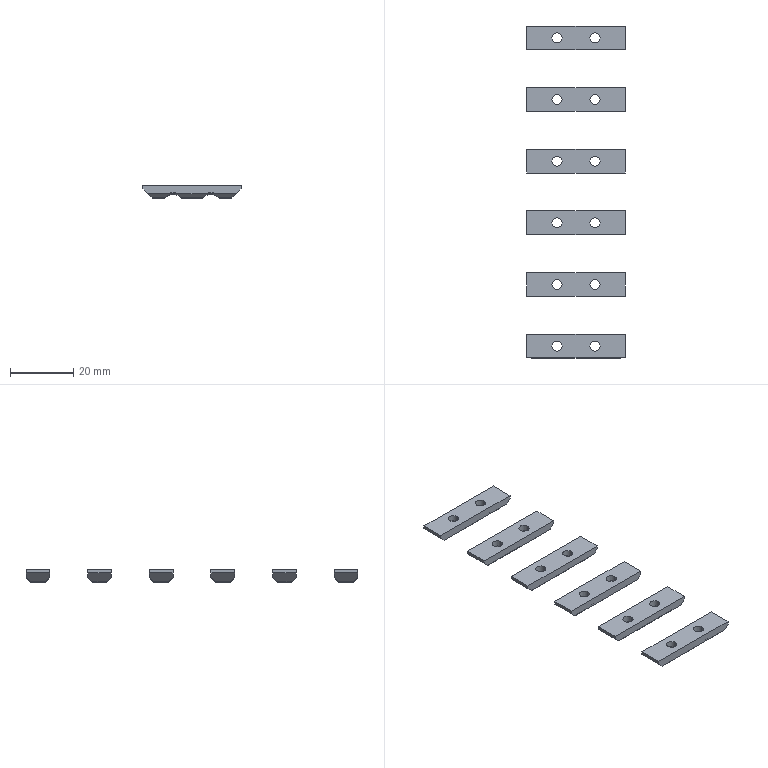NC program | NX | posted with a generic post | part box 31 x 105 x 4 mm
Lines 12431 to 12738 of 12738:
(ZLEVEL_PROFILE_1_COPY , TOOL : D10JING)
N24788 T14 M6
N24790 G54
N24792 G17 G0 G90 X44.871 Y20.5 S9500 M3
N24794 G43 Z30. H14
N24796 Z-1.9
N24798 G94 G1 X53.049 Z-2.329 F1000.
N24800 X54.364 Y20.172 Z-2.4
N24802 X55.545 Y19.504 Z-2.471
N24804 X56.504 Y18.545 Z-2.542
N24806 X57.172 Y17.364 Z-2.613
N24808 X57.5 Y16.049 Z-2.684
N24810 Y0. Z-3.525
N24812 Y-15.5 F1200.
N24814 G2 X52.5 Y-20.5 R5.
N24816 G1 X45.
N24818 G2 X40. Y-15.5 R5.
N24820 G1 Y15.5
N24822 G2 X45. Y20.5 R5.
N24824 G1 X52.5
N24826 G2 X57.5 Y15.5 R5.
N24828 G1 Y0.
N24830 Y-7.161 Z-3.65
N24832 Y-15.5
N24834 G2 X52.5 Y-20.5 R5.
N24836 G1 X45.
N24838 G2 X40. Y-15.5 R5.
N24840 G1 Y15.5
N24842 G2 X45. Y20.5 R5.
N24844 G1 X52.5
N24846 G2 X57.5 Y15.5 R5.
N24848 G1 Y0.
N24850 Y-7.161 Z-3.775
N24852 Y-15.5
N24854 G2 X52.5 Y-20.5 R5.
N24856 G1 X45.
N24858 G2 X40. Y-15.5 R5.
N24860 G1 Y15.5
N24862 G2 X45. Y20.5 R5.
N24864 G1 X52.5
N24866 G2 X57.5 Y15.5 R5.
N24868 G1 Y0.
N24870 Y-7.161 Z-3.9
N24872 Y-15.5
N24874 G2 X52.5 Y-20.5 R5.
N24876 G1 X45.
N24878 G2 X40. Y-15.5 R5.
N24880 G1 Y15.5
N24882 G2 X45. Y20.5 R5.
N24884 G1 X52.5
N24886 G2 X57.5 Y15.5 R5.
N24888 G1 Y-7.161
N24890 Z-2.4
N24892 G0 Z30.
N24894 X-44.871 Y-20.5
N24896 Z-1.9
N24898 G1 X-53.049 Z-2.329 F1000.
N24900 X-54.364 Y-20.172 Z-2.4
N24902 X-55.545 Y-19.504 Z-2.471
N24904 X-56.504 Y-18.545 Z-2.542
N24906 X-57.172 Y-17.364 Z-2.613
N24908 X-57.5 Y-16.049 Z-2.684
N24910 Y0. Z-3.525
N24912 Y15.5 F1200.
N24914 G2 X-52.5 Y20.5 R5.
N24916 G1 X-45.
N24918 G2 X-40. Y15.5 R5.
N24920 G1 Y-15.5
N24922 G2 X-45. Y-20.5 R5.
N24924 G1 X-52.5
N24926 G2 X-57.5 Y-15.5 R5.
N24928 G1 Y0.
N24930 Y7.161 Z-3.65
N24932 Y15.5
N24934 G2 X-52.5 Y20.5 R5.
N24936 G1 X-45.
N24938 G2 X-40. Y15.5 R5.
N24940 G1 Y-15.5
N24942 G2 X-45. Y-20.5 R5.
N24944 G1 X-52.5
N24946 G2 X-57.5 Y-15.5 R5.
N24948 G1 Y0.
N24950 Y7.161 Z-3.775
N24952 Y15.5
N24954 G2 X-52.5 Y20.5 R5.
N24956 G1 X-45.
N24958 G2 X-40. Y15.5 R5.
N24960 G1 Y-15.5
N24962 G2 X-45. Y-20.5 R5.
N24964 G1 X-52.5
N24966 G2 X-57.5 Y-15.5 R5.
N24968 G1 Y0.
N24970 Y7.161 Z-3.9
N24972 Y15.5
N24974 G2 X-52.5 Y20.5 R5.
N24976 G1 X-45.
N24978 G2 X-40. Y15.5 R5.
N24980 G1 Y-15.5
N24982 G2 X-45. Y-20.5 R5.
N24984 G1 X-52.5
N24986 G2 X-57.5 Y-15.5 R5.
N24988 G1 Y7.161
N24990 Z-2.4
N24992 G0 Z30.
N24994 X-25.371 Y-20.5
N24996 Z-1.9
N24998 G1 X-33.549 Z-2.329 F1000.
N25000 X-34.864 Y-20.172 Z-2.4
N25002 X-36.045 Y-19.504 Z-2.471
N25004 X-37.004 Y-18.545 Z-2.542
N25006 X-37.672 Y-17.364 Z-2.613
N25008 X-38. Y-16.049 Z-2.684
N25010 Y0. Z-3.525
N25012 Y15.5 F1200.
N25014 G2 X-33. Y20.5 R5.
N25016 G1 X-25.5
N25018 G2 X-20.5 Y15.5 R5.
N25020 G1 Y-15.5
N25022 G2 X-25.5 Y-20.5 R5.
N25024 G1 X-33.
N25026 G2 X-38. Y-15.5 R5.
N25028 G1 Y0.
N25030 Y7.161 Z-3.65
N25032 Y15.5
N25034 G2 X-33. Y20.5 R5.
N25036 G1 X-25.5
N25038 G2 X-20.5 Y15.5 R5.
N25040 G1 Y-15.5
N25042 G2 X-25.5 Y-20.5 R5.
N25044 G1 X-33.
N25046 G2 X-38. Y-15.5 R5.
N25048 G1 Y0.
N25050 Y7.161 Z-3.775
N25052 Y15.5
N25054 G2 X-33. Y20.5 R5.
N25056 G1 X-25.5
N25058 G2 X-20.5 Y15.5 R5.
N25060 G1 Y-15.5
N25062 G2 X-25.5 Y-20.5 R5.
N25064 G1 X-33.
N25066 G2 X-38. Y-15.5 R5.
N25068 G1 Y0.
N25070 Y7.161 Z-3.9
N25072 Y15.5
N25074 G2 X-33. Y20.5 R5.
N25076 G1 X-25.5
N25078 G2 X-20.5 Y15.5 R5.
N25080 G1 Y-15.5
N25082 G2 X-25.5 Y-20.5 R5.
N25084 G1 X-33.
N25086 G2 X-38. Y-15.5 R5.
N25088 G1 Y7.161
N25090 Z-2.4
N25092 G0 Z30.
N25094 X-5.871 Y-20.5
N25096 Z-1.9
N25098 G1 X-14.049 Z-2.329 F1000.
N25100 X-15.364 Y-20.172 Z-2.4
N25102 X-16.545 Y-19.504 Z-2.471
N25104 X-17.504 Y-18.545 Z-2.542
N25106 X-18.172 Y-17.364 Z-2.613
N25108 X-18.5 Y-16.049 Z-2.684
N25110 Y0. Z-3.525
N25112 Y15.5 F1200.
N25114 G2 X-13.5 Y20.5 R5.
N25116 G1 X-6.
N25118 G2 X-1. Y15.5 R5.
N25120 G1 Y-15.5
N25122 G2 X-6. Y-20.5 R5.
N25124 G1 X-13.5
N25126 G2 X-18.5 Y-15.5 R5.
N25128 G1 Y0.
N25130 Y7.161 Z-3.65
N25132 Y15.5
N25134 G2 X-13.5 Y20.5 R5.
N25136 G1 X-6.
N25138 G2 X-1. Y15.5 R5.
N25140 G1 Y-15.5
N25142 G2 X-6. Y-20.5 R5.
N25144 G1 X-13.5
N25146 G2 X-18.5 Y-15.5 R5.
N25148 G1 Y0.
N25150 Y7.161 Z-3.775
N25152 Y15.5
N25154 G2 X-13.5 Y20.5 R5.
N25156 G1 X-6.
N25158 G2 X-1. Y15.5 R5.
N25160 G1 Y-15.5
N25162 G2 X-6. Y-20.5 R5.
N25164 G1 X-13.5
N25166 G2 X-18.5 Y-15.5 R5.
N25168 G1 Y0.
N25170 Y7.161 Z-3.9
N25172 Y15.5
N25174 G2 X-13.5 Y20.5 R5.
N25176 G1 X-6.
N25178 G2 X-1. Y15.5 R5.
N25180 G1 Y-15.5
N25182 G2 X-6. Y-20.5 R5.
N25184 G1 X-13.5
N25186 G2 X-18.5 Y-15.5 R5.
N25188 G1 Y7.161
N25190 Z-2.4
N25192 G0 Z30.
N25194 X13.629 Y-20.5
N25196 Z-1.9
N25198 G1 X5.451 Z-2.329 F1000.
N25200 X4.136 Y-20.172 Z-2.4
N25202 X2.955 Y-19.504 Z-2.471
N25204 X1.996 Y-18.545 Z-2.542
N25206 X1.328 Y-17.364 Z-2.613
N25208 X1. Y-16.049 Z-2.684
N25210 Y0. Z-3.525
N25212 Y15.5 F1200.
N25214 G2 X6. Y20.5 R5.
N25216 G1 X13.5
N25218 G2 X18.5 Y15.5 R5.
N25220 G1 Y-15.5
N25222 G2 X13.5 Y-20.5 R5.
N25224 G1 X6.
N25226 G2 X1. Y-15.5 R5.
N25228 G1 Y0.
N25230 Y7.161 Z-3.65
N25232 Y15.5
N25234 G2 X6. Y20.5 R5.
N25236 G1 X13.5
N25238 G2 X18.5 Y15.5 R5.
N25240 G1 Y-15.5
N25242 G2 X13.5 Y-20.5 R5.
N25244 G1 X6.
N25246 G2 X1. Y-15.5 R5.
N25248 G1 Y0.
N25250 Y7.161 Z-3.775
N25252 Y15.5
N25254 G2 X6. Y20.5 R5.
N25256 G1 X13.5
N25258 G2 X18.5 Y15.5 R5.
N25260 G1 Y-15.5
N25262 G2 X13.5 Y-20.5 R5.
N25264 G1 X6.
N25266 G2 X1. Y-15.5 R5.
N25268 G1 Y0.
N25270 Y7.161 Z-3.9
N25272 Y15.5
N25274 G2 X6. Y20.5 R5.
N25276 G1 X13.5
N25278 G2 X18.5 Y15.5 R5.
N25280 G1 Y-15.5
N25282 G2 X13.5 Y-20.5 R5.
N25284 G1 X6.
N25286 G2 X1. Y-15.5 R5.
N25288 G1 Y7.161
N25290 Z-2.4
N25292 G0 Z30.
N25294 X33.129 Y-20.5
N25296 Z-1.9
N25298 G1 X24.951 Z-2.329 F1000.
N25300 X23.636 Y-20.172 Z-2.4
N25302 X22.455 Y-19.504 Z-2.471
N25304 X21.496 Y-18.545 Z-2.542
N25306 X20.828 Y-17.364 Z-2.613
N25308 X20.5 Y-16.049 Z-2.684
N25310 Y0. Z-3.525
N25312 Y15.5 F1200.
N25314 G2 X25.5 Y20.5 R5.
N25316 G1 X33.
N25318 G2 X38. Y15.5 R5.
N25320 G1 Y-15.5
N25322 G2 X33. Y-20.5 R5.
N25324 G1 X25.5
N25326 G2 X20.5 Y-15.5 R5.
N25328 G1 Y0.
N25330 Y7.161 Z-3.65
N25332 Y15.5
N25334 G2 X25.5 Y20.5 R5.
N25336 G1 X33.
N25338 G2 X38. Y15.5 R5.
N25340 G1 Y-15.5
N25342 G2 X33. Y-20.5 R5.
N25344 G1 X25.5
N25346 G2 X20.5 Y-15.5 R5.
N25348 G1 Y0.
N25350 Y7.161 Z-3.775
N25352 Y15.5
N25354 G2 X25.5 Y20.5 R5.
N25356 G1 X33.
N25358 G2 X38. Y15.5 R5.
N25360 G1 Y-15.5
N25362 G2 X33. Y-20.5 R5.
N25364 G1 X25.5
N25366 G2 X20.5 Y-15.5 R5.
N25368 G1 Y0.
N25370 Y7.161 Z-3.9
N25372 Y15.5
N25374 G2 X25.5 Y20.5 R5.
N25376 G1 X33.
N25378 G2 X38. Y15.5 R5.
N25380 G1 Y-15.5
N25382 G2 X33. Y-20.5 R5.
N25384 G1 X25.5
N25386 G2 X20.5 Y-15.5 R5.
N25388 G1 Y7.161
N25390 Z-2.4
N25392 G0 Z30.
N25394 M5
N25396 M2